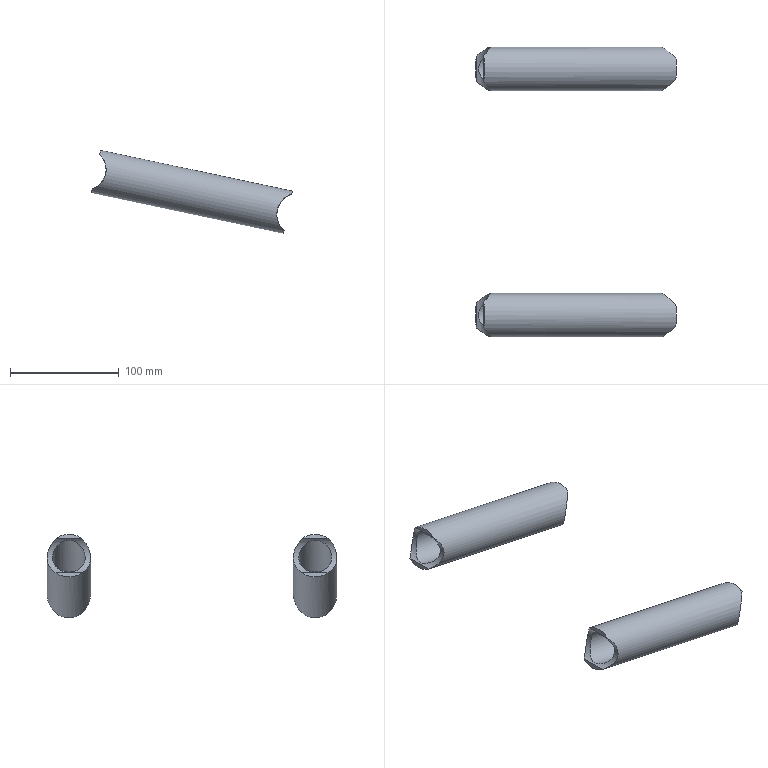Part | STEP file | HL4GZ-1.862.057 (lower swing arm weldment) | 2 solids | 16 faces | box 184.383 x 266 x 76.55 mm | volume 187249 mm3 | cylinder 8 | plane 8 | commonest cylinder face diameters 40 x4 30 x2 38 x2